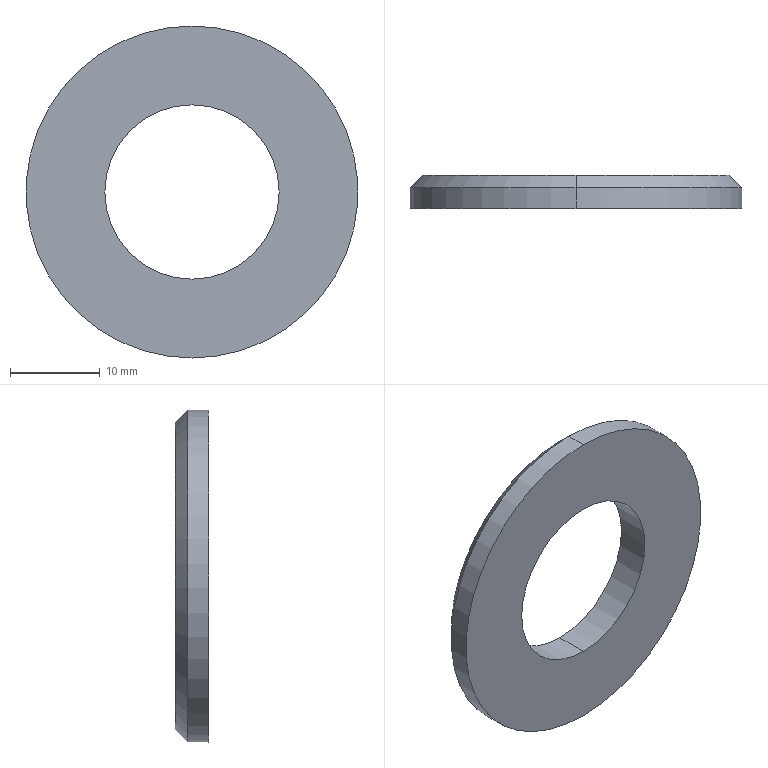Part | SolidWorks | features BaseBody 1 | 1 solid | 8 faces | box 36.923 x 3.692 x 36.923 mm | volume 2755 mm3 | cylinder 4 | cone 2 | plane 2 | commonest cylinder face diameters 19.385 x2 36.923 x2
STEP:
#1=CARTESIAN_POINT('',(57.247,375.5,255.846));
#2=VERTEX_POINT('',#1);
#3=CARTESIAN_POINT('',(57.247,375.5,236.462));
#4=VERTEX_POINT('',#3);
#5=CARTESIAN_POINT('',(57.247,375.5,246.154));
#6=DIRECTION('',(0.,-1.,0.));
#7=DIRECTION('',(0.,0.,-1.));
#8=AXIS2_PLACEMENT_3D('',#5,#6,#7);
#9=CIRCLE('',#8,9.692);
#10=EDGE_CURVE('',#2,#4,#9,.T.);
#11=ORIENTED_EDGE('',*,*,#10,.F.);
#12=CARTESIAN_POINT('',(57.247,371.808,255.846));
#13=VERTEX_POINT('',#12);
#14=CARTESIAN_POINT('',(57.247,375.5,255.846));
#15=DIRECTION('',(0.,-1.,0.));
#16=VECTOR('',#15,1000.);
#17=LINE('',#14,#16);
#18=EDGE_CURVE('',#2,#13,#17,.T.);
#19=ORIENTED_EDGE('',*,*,#18,.T.);
#20=CARTESIAN_POINT('',(57.247,371.808,236.462));
#21=VERTEX_POINT('',#20);
#22=CARTESIAN_POINT('',(57.247,371.808,246.154));
#23=DIRECTION('',(0.,1.,0.));
#24=DIRECTION('',(0.,0.,-1.));
#25=AXIS2_PLACEMENT_3D('',#22,#23,#24);
#26=CIRCLE('',#25,9.692);
#27=EDGE_CURVE('',#21,#13,#26,.T.);
#28=ORIENTED_EDGE('',*,*,#27,.F.);
#29=CARTESIAN_POINT('',(57.247,375.5,236.462));
#30=DIRECTION('',(0.,-1.,0.));
#31=VECTOR('',#30,1000.);
#32=LINE('',#29,#31);
#33=EDGE_CURVE('',#4,#21,#32,.T.);
#34=ORIENTED_EDGE('',*,*,#33,.F.);
#35=EDGE_LOOP('',(#11,#19,#28,#34));
#36=FACE_OUTER_BOUND('',#35,.T.);
#37=CARTESIAN_POINT('',(57.247,375.5,246.154));
#38=DIRECTION('',(0.,-1.,0.));
#39=DIRECTION('',(0.,0.,-1.));
#40=AXIS2_PLACEMENT_3D('',#37,#38,#39);
#41=CYLINDRICAL_SURFACE('',#40,9.692);
#42=ADVANCED_FACE('',(#36),#41,.F.);
#43=CARTESIAN_POINT('',(57.247,374.115,227.692));
#44=VERTEX_POINT('',#43);
#45=CARTESIAN_POINT('',(57.247,374.115,264.615));
#46=VERTEX_POINT('',#45);
#47=CARTESIAN_POINT('',(57.247,374.115,246.154));
#48=DIRECTION('',(0.,-1.,0.));
#49=DIRECTION('',(0.,0.,-1.));
#50=AXIS2_PLACEMENT_3D('',#47,#48,#49);
#51=CIRCLE('',#50,18.462);
#52=EDGE_CURVE('',#44,#46,#51,.T.);
#53=ORIENTED_EDGE('',*,*,#52,.T.);
#54=CARTESIAN_POINT('',(57.247,371.808,264.615));
#55=VERTEX_POINT('',#54);
#56=CARTESIAN_POINT('',(57.247,375.5,264.615));
#57=DIRECTION('',(0.,-1.,0.));
#58=VECTOR('',#57,1000.);
#59=LINE('',#56,#58);
#60=EDGE_CURVE('',#46,#55,#59,.T.);
#61=ORIENTED_EDGE('',*,*,#60,.T.);
#62=CARTESIAN_POINT('',(57.247,371.808,227.692));
#63=VERTEX_POINT('',#62);
#64=CARTESIAN_POINT('',(57.247,371.808,246.154));
#65=DIRECTION('',(0.,-1.,0.));
#66=DIRECTION('',(0.,0.,-1.));
#67=AXIS2_PLACEMENT_3D('',#64,#65,#66);
#68=CIRCLE('',#67,18.462);
#69=EDGE_CURVE('',#63,#55,#68,.T.);
#70=ORIENTED_EDGE('',*,*,#69,.F.);
#71=CARTESIAN_POINT('',(57.247,375.5,227.692));
#72=DIRECTION('',(0.,-1.,0.));
#73=VECTOR('',#72,1000.);
#74=LINE('',#71,#73);
#75=EDGE_CURVE('',#44,#63,#74,.T.);
#76=ORIENTED_EDGE('',*,*,#75,.F.);
#77=EDGE_LOOP('',(#53,#61,#70,#76));
#78=FACE_OUTER_BOUND('',#77,.T.);
#79=CARTESIAN_POINT('',(57.247,375.5,246.154));
#80=DIRECTION('',(0.,-1.,0.));
#81=DIRECTION('',(0.,0.,-1.));
#82=AXIS2_PLACEMENT_3D('',#79,#80,#81);
#83=CYLINDRICAL_SURFACE('',#82,18.462);
#84=ADVANCED_FACE('',(#78),#83,.T.);
#85=CARTESIAN_POINT('',(57.247,375.5,263.231));
#86=VERTEX_POINT('',#85);
#87=CARTESIAN_POINT('',(57.247,375.5,229.077));
#88=VERTEX_POINT('',#87);
#89=CARTESIAN_POINT('',(57.247,375.5,246.154));
#90=DIRECTION('',(0.,1.,0.));
#91=DIRECTION('',(0.,0.,-1.));
#92=AXIS2_PLACEMENT_3D('',#89,#90,#91);
#93=CIRCLE('',#92,17.077);
#94=EDGE_CURVE('',#86,#88,#93,.T.);
#95=ORIENTED_EDGE('',*,*,#94,.F.);
#96=CARTESIAN_POINT('',(57.247,374.115,264.615));
#97=DIRECTION('',(0.,-0.7071,0.7071));
#98=VECTOR('',#97,1000.);
#99=LINE('',#96,#98);
#100=EDGE_CURVE('',#86,#46,#99,.T.);
#101=ORIENTED_EDGE('',*,*,#100,.T.);
#102=ORIENTED_EDGE('',*,*,#52,.F.);
#103=CARTESIAN_POINT('',(57.247,374.115,227.692));
#104=DIRECTION('',(0.,-0.7071,-0.7071));
#105=VECTOR('',#104,1000.);
#106=LINE('',#103,#105);
#107=EDGE_CURVE('',#88,#44,#106,.T.);
#108=ORIENTED_EDGE('',*,*,#107,.F.);
#109=EDGE_LOOP('',(#95,#101,#102,#108));
#110=FACE_OUTER_BOUND('',#109,.T.);
#111=CARTESIAN_POINT('',(57.247,374.115,246.154));
#112=DIRECTION('',(0.,-1.,0.));
#113=DIRECTION('',(0.,0.,-1.));
#114=AXIS2_PLACEMENT_3D('',#111,#112,#113);
#115=CONICAL_SURFACE('',#114,18.462,0.7854);
#116=ADVANCED_FACE('',(#110),#115,.T.);
#117=ORIENTED_EDGE('',*,*,#27,.T.);
#118=CARTESIAN_POINT('',(57.247,371.808,246.154));
#119=DIRECTION('',(0.,1.,0.));
#120=DIRECTION('',(0.,0.,-1.));
#121=AXIS2_PLACEMENT_3D('',#118,#119,#120);
#122=CIRCLE('',#121,9.692);
#123=EDGE_CURVE('',#13,#21,#122,.T.);
#124=ORIENTED_EDGE('',*,*,#123,.T.);
#125=EDGE_LOOP('',(#117,#124));
#126=FACE_BOUND('',#125,.T.);
#127=ORIENTED_EDGE('',*,*,#69,.T.);
#128=CARTESIAN_POINT('',(57.247,371.808,246.154));
#129=DIRECTION('',(0.,-1.,0.));
#130=DIRECTION('',(0.,0.,-1.));
#131=AXIS2_PLACEMENT_3D('',#128,#129,#130);
#132=CIRCLE('',#131,18.462);
#133=EDGE_CURVE('',#55,#63,#132,.T.);
#134=ORIENTED_EDGE('',*,*,#133,.T.);
#135=EDGE_LOOP('',(#127,#134));
#136=FACE_OUTER_BOUND('',#135,.T.);
#137=CARTESIAN_POINT('',(38.785,371.808,246.154));
#138=DIRECTION('',(0.,-1.,0.));
#139=DIRECTION('',(0.,0.,-1.));
#140=AXIS2_PLACEMENT_3D('',#137,#138,#139);
#141=PLANE('',#140);
#142=ADVANCED_FACE('',(#126,#136),#141,.T.);
#143=ORIENTED_EDGE('',*,*,#18,.F.);
#144=CARTESIAN_POINT('',(57.247,375.5,246.154));
#145=DIRECTION('',(0.,-1.,0.));
#146=DIRECTION('',(0.,0.,-1.));
#147=AXIS2_PLACEMENT_3D('',#144,#145,#146);
#148=CIRCLE('',#147,9.692);
#149=EDGE_CURVE('',#4,#2,#148,.T.);
#150=ORIENTED_EDGE('',*,*,#149,.F.);
#151=ORIENTED_EDGE('',*,*,#33,.T.);
#152=ORIENTED_EDGE('',*,*,#123,.F.);
#153=EDGE_LOOP('',(#143,#150,#151,#152));
#154=FACE_OUTER_BOUND('',#153,.T.);
#155=CARTESIAN_POINT('',(57.247,375.5,246.154));
#156=DIRECTION('',(0.,-1.,0.));
#157=DIRECTION('',(0.,0.,-1.));
#158=AXIS2_PLACEMENT_3D('',#155,#156,#157);
#159=CYLINDRICAL_SURFACE('',#158,9.692);
#160=ADVANCED_FACE('',(#154),#159,.F.);
#161=ORIENTED_EDGE('',*,*,#60,.F.);
#162=CARTESIAN_POINT('',(57.247,374.115,246.154));
#163=DIRECTION('',(0.,-1.,0.));
#164=DIRECTION('',(0.,0.,-1.));
#165=AXIS2_PLACEMENT_3D('',#162,#163,#164);
#166=CIRCLE('',#165,18.462);
#167=EDGE_CURVE('',#46,#44,#166,.T.);
#168=ORIENTED_EDGE('',*,*,#167,.T.);
#169=ORIENTED_EDGE('',*,*,#75,.T.);
#170=ORIENTED_EDGE('',*,*,#133,.F.);
#171=EDGE_LOOP('',(#161,#168,#169,#170));
#172=FACE_OUTER_BOUND('',#171,.T.);
#173=CARTESIAN_POINT('',(57.247,375.5,246.154));
#174=DIRECTION('',(0.,-1.,0.));
#175=DIRECTION('',(0.,0.,-1.));
#176=AXIS2_PLACEMENT_3D('',#173,#174,#175);
#177=CYLINDRICAL_SURFACE('',#176,18.462);
#178=ADVANCED_FACE('',(#172),#177,.T.);
#179=ORIENTED_EDGE('',*,*,#149,.T.);
#180=ORIENTED_EDGE('',*,*,#10,.T.);
#181=EDGE_LOOP('',(#179,#180));
#182=FACE_BOUND('',#181,.T.);
#183=CARTESIAN_POINT('',(57.247,375.5,246.154));
#184=DIRECTION('',(0.,1.,0.));
#185=DIRECTION('',(0.,0.,-1.));
#186=AXIS2_PLACEMENT_3D('',#183,#184,#185);
#187=CIRCLE('',#186,17.077);
#188=EDGE_CURVE('',#88,#86,#187,.T.);
#189=ORIENTED_EDGE('',*,*,#188,.T.);
#190=ORIENTED_EDGE('',*,*,#94,.T.);
#191=EDGE_LOOP('',(#189,#190));
#192=FACE_OUTER_BOUND('',#191,.T.);
#193=CARTESIAN_POINT('',(47.554,375.5,246.154));
#194=DIRECTION('',(0.,1.,0.));
#195=DIRECTION('',(0.,0.,1.));
#196=AXIS2_PLACEMENT_3D('',#193,#194,#195);
#197=PLANE('',#196);
#198=ADVANCED_FACE('',(#182,#192),#197,.T.);
#199=ORIENTED_EDGE('',*,*,#100,.F.);
#200=ORIENTED_EDGE('',*,*,#188,.F.);
#201=ORIENTED_EDGE('',*,*,#107,.T.);
#202=ORIENTED_EDGE('',*,*,#167,.F.);
#203=EDGE_LOOP('',(#199,#200,#201,#202));
#204=FACE_OUTER_BOUND('',#203,.T.);
#205=CARTESIAN_POINT('',(57.247,374.115,246.154));
#206=DIRECTION('',(0.,-1.,0.));
#207=DIRECTION('',(0.,0.,-1.));
#208=AXIS2_PLACEMENT_3D('',#205,#206,#207);
#209=CONICAL_SURFACE('',#208,18.462,0.7854);
#210=ADVANCED_FACE('',(#204),#209,.T.);
#211=CLOSED_SHELL('',(#42,#84,#116,#142,#160,#178,#198,#210));
#212=MANIFOLD_SOLID_BREP('',#211);
#213=CARTESIAN_POINT('',(0.,0.,0.));
#214=DIRECTION('',(0.,0.,1.));
#215=DIRECTION('',(1.,0.,0.));
#216=AXIS2_PLACEMENT_3D('',#213,#214,#215);
#217=(LENGTH_UNIT()NAMED_UNIT(*)SI_UNIT(.MILLI.,.METRE.));
#218=UNCERTAINTY_MEASURE_WITH_UNIT(LENGTH_MEASURE(0.00001),#217,'','');
#219=(NAMED_UNIT(*)PLANE_ANGLE_UNIT()SI_UNIT($,.RADIAN.));
#220=(NAMED_UNIT(*)SI_UNIT($,.STERADIAN.)SOLID_ANGLE_UNIT());
#221=(GEOMETRIC_REPRESENTATION_CONTEXT(3)GLOBAL_UNCERTAINTY_ASSIGNED_CONTEXT((#218))GLOBAL_UNIT_ASSIGNED_CONTEXT((#217,#219,#220))REPRESENTATION_CONTEXT('',''));
#222=ADVANCED_BREP_SHAPE_REPRESENTATION('',(#212,#216),#221);